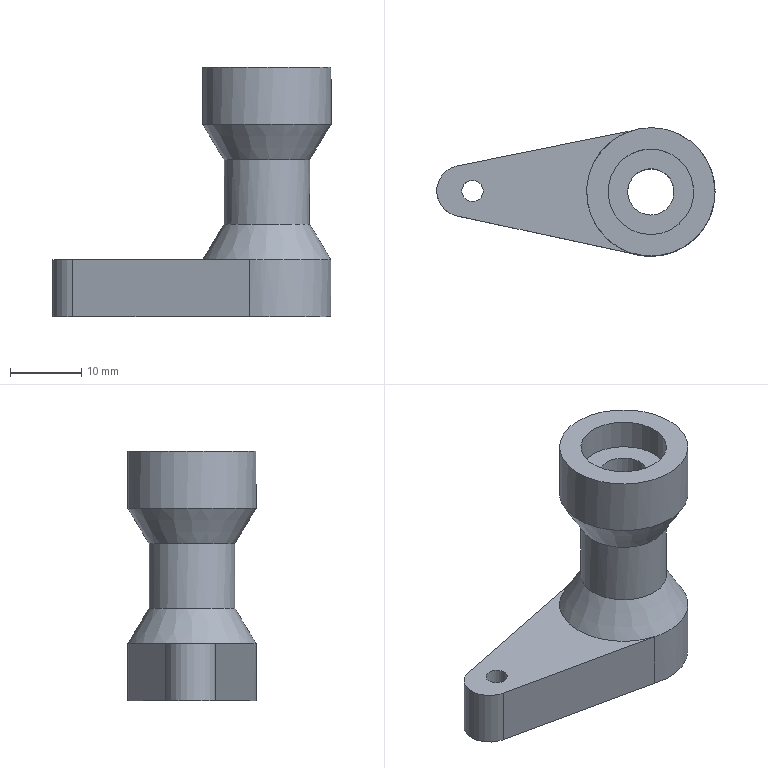Part | STEP file | Dodanie-wyci_gni_cie1_2 | 1 solid | 18 faces | box 38.999 x 17.999 x 35 mm | volume 6844 mm3 | cylinder 9 | plane 7 | cone 2 | commonest cylinder face diameters 11.999 x3 17.999 x3 3 x1 6.499 x1 7.151 x1
STEP:
#1=CARTESIAN_POINT('',(0.,0.,0.));
#2=DIRECTION('',(0.,0.,1.));
#3=DIRECTION('',(1.,0.,0.));
#4=AXIS2_PLACEMENT_3D('',#1,#2,#3);
#5=CARTESIAN_POINT('',(-38.722,78.388,-127.298));
#6=VERTEX_POINT('',#5);
#7=CARTESIAN_POINT('',(-38.744,75.138,-127.298));
#8=DIRECTION('',(0.,0.,1.));
#9=DIRECTION('',(0.006749,1.,0.));
#10=AXIS2_PLACEMENT_3D('',#7,#8,#9);
#11=CIRCLE('',#10,3.25);
#12=CARTESIAN_POINT('',(-38.744,75.138,-127.298));
#13=DIRECTION('',(0.,0.,1.));
#14=DIRECTION('',(0.006749,1.,0.));
#15=AXIS2_PLACEMENT_3D('',#12,#13,#14);
#16=CYLINDRICAL_SURFACE('',#15,3.25);
#17=CARTESIAN_POINT('',(0.,0.));
#18=DIRECTION('',(1.,0.));
#19=VECTOR('',#18,1.);
#20=LINE('',#17,#19);
#21=(GEOMETRIC_REPRESENTATION_CONTEXT(2)PARAMETRIC_REPRESENTATION_CONTEXT()REPRESENTATION_CONTEXT('',''));
#22=DEFINITIONAL_REPRESENTATION('',(#20),#21);
#23=PCURVE('',#16,#22);
#24=CARTESIAN_POINT('',(-38.744,75.138,-127.298));
#25=DIRECTION('',(0.,0.,-1.));
#26=DIRECTION('',(-0.006749,-1.,0.));
#27=AXIS2_PLACEMENT_3D('',#24,#25,#26);
#28=PLANE('',#27);
#29=CARTESIAN_POINT('',(-3.25,0.));
#30=CARTESIAN_POINT('',(-3.25,5.629));
#31=CARTESIAN_POINT('',(1.625,2.814));
#32=CARTESIAN_POINT('',(6.499,0.));
#33=CARTESIAN_POINT('',(1.625,-2.814));
#34=CARTESIAN_POINT('',(-3.25,-5.629));
#35=CARTESIAN_POINT('',(-3.25,0.));
#36=(BOUNDED_CURVE()B_SPLINE_CURVE(2,(#29,#30,#31,#32,#33,#34,#35),.UNSPECIFIED.,.T.,.F.)B_SPLINE_CURVE_WITH_KNOTS((1,2,2,2,2,1),(-2.094,0.,2.094,4.189,6.283,8.378),.UNSPECIFIED.)CURVE()GEOMETRIC_REPRESENTATION_ITEM()RATIONAL_B_SPLINE_CURVE((1.,0.5,1.,0.5,1.,0.5,1.))REPRESENTATION_ITEM(''));
#37=(GEOMETRIC_REPRESENTATION_CONTEXT(2)PARAMETRIC_REPRESENTATION_CONTEXT()REPRESENTATION_CONTEXT('',''));
#38=DEFINITIONAL_REPRESENTATION('',(#36),#37);
#39=PCURVE('',#28,#38);
#40=SURFACE_CURVE('',#11,(#23,#39),.PCURVE_S1.);
#41=EDGE_CURVE('',#6,#6,#40,.T.);
#42=ORIENTED_EDGE('',*,*,#41,.T.);
#43=CARTESIAN_POINT('',(-38.722,78.388,-100.698));
#44=VERTEX_POINT('',#43);
#45=CARTESIAN_POINT('',(-38.722,78.388,-100.698));
#46=DIRECTION('',(0.,0.,-1.));
#47=VECTOR('',#46,1.);
#48=LINE('',#45,#47);
#49=CARTESIAN_POINT('',(6.283,26.6));
#50=DIRECTION('',(0.,-1.));
#51=VECTOR('',#50,1.);
#52=LINE('',#49,#51);
#53=(GEOMETRIC_REPRESENTATION_CONTEXT(2)PARAMETRIC_REPRESENTATION_CONTEXT()REPRESENTATION_CONTEXT('',''));
#54=DEFINITIONAL_REPRESENTATION('',(#52),#53);
#55=PCURVE('',#16,#54);
#56=CARTESIAN_POINT('',(0.,26.6));
#57=DIRECTION('',(0.,-1.));
#58=VECTOR('',#57,1.);
#59=LINE('',#56,#58);
#60=(GEOMETRIC_REPRESENTATION_CONTEXT(2)PARAMETRIC_REPRESENTATION_CONTEXT()REPRESENTATION_CONTEXT('',''));
#61=DEFINITIONAL_REPRESENTATION('',(#59),#60);
#62=PCURVE('',#16,#61);
#63=SEAM_CURVE('',#48,(#55,#62),.PCURVE_S1.);
#64=EDGE_CURVE('',#44,#6,#63,.T.);
#65=ORIENTED_EDGE('',*,*,#64,.F.);
#66=CARTESIAN_POINT('',(-38.744,75.138,-100.698));
#67=DIRECTION('',(0.,0.,-1.));
#68=DIRECTION('',(0.006749,1.,0.));
#69=AXIS2_PLACEMENT_3D('',#66,#67,#68);
#70=CIRCLE('',#69,3.25);
#71=CARTESIAN_POINT('',(6.283,26.6));
#72=DIRECTION('',(-1.,0.));
#73=VECTOR('',#72,1.);
#74=LINE('',#71,#73);
#75=(GEOMETRIC_REPRESENTATION_CONTEXT(2)PARAMETRIC_REPRESENTATION_CONTEXT()REPRESENTATION_CONTEXT('',''));
#76=DEFINITIONAL_REPRESENTATION('',(#74),#75);
#77=PCURVE('',#16,#76);
#78=CARTESIAN_POINT('',(-38.744,75.138,-100.698));
#79=DIRECTION('',(0.,0.,-1.));
#80=DIRECTION('',(-0.006749,-1.,0.));
#81=AXIS2_PLACEMENT_3D('',#78,#79,#80);
#82=PLANE('',#81);
#83=CARTESIAN_POINT('',(0.,0.));
#84=DIRECTION('',(-1.,0.));
#85=AXIS2_PLACEMENT_2D('',#83,#84);
#86=CIRCLE('',#85,3.25);
#87=(GEOMETRIC_REPRESENTATION_CONTEXT(2)PARAMETRIC_REPRESENTATION_CONTEXT()REPRESENTATION_CONTEXT('',''));
#88=DEFINITIONAL_REPRESENTATION('',(#86),#87);
#89=PCURVE('',#82,#88);
#90=SURFACE_CURVE('',#70,(#77,#89),.PCURVE_S1.);
#91=EDGE_CURVE('',#44,#44,#90,.T.);
#92=ORIENTED_EDGE('',*,*,#91,.T.);
#93=ORIENTED_EDGE('',*,*,#64,.T.);
#94=EDGE_LOOP('',(#42,#65,#92,#93));
#95=FACE_BOUND('',#94,.F.);
#96=ADVANCED_FACE('',(#95),#16,.F.);
#97=CARTESIAN_POINT('',(-38.704,81.138,-131.498));
#98=VERTEX_POINT('',#97);
#99=CARTESIAN_POINT('',(-38.744,75.138,-131.498));
#100=DIRECTION('',(0.,0.,1.));
#101=DIRECTION('',(0.006749,1.,0.));
#102=AXIS2_PLACEMENT_3D('',#99,#100,#101);
#103=CIRCLE('',#102,6.);
#104=CARTESIAN_POINT('',(-38.744,75.138,-131.498));
#105=DIRECTION('',(0.,0.,1.));
#106=DIRECTION('',(0.006749,1.,0.));
#107=AXIS2_PLACEMENT_3D('',#104,#105,#106);
#108=CYLINDRICAL_SURFACE('',#107,6.);
#109=CARTESIAN_POINT('',(0.,0.));
#110=DIRECTION('',(1.,0.));
#111=VECTOR('',#110,1.);
#112=LINE('',#109,#111);
#113=(GEOMETRIC_REPRESENTATION_CONTEXT(2)PARAMETRIC_REPRESENTATION_CONTEXT()REPRESENTATION_CONTEXT('',''));
#114=DEFINITIONAL_REPRESENTATION('',(#112),#113);
#115=PCURVE('',#108,#114);
#116=CARTESIAN_POINT('',(-49.244,75.209,-131.498));
#117=DIRECTION('',(0.,0.,-1.));
#118=DIRECTION('',(-0.006749,-1.,0.));
#119=AXIS2_PLACEMENT_3D('',#116,#117,#118);
#120=PLANE('',#119);
#121=CARTESIAN_POINT('',(-6.,-10.5));
#122=CARTESIAN_POINT('',(-6.,-0.1086));
#123=CARTESIAN_POINT('',(3.,-5.304));
#124=CARTESIAN_POINT('',(11.999,-10.5));
#125=CARTESIAN_POINT('',(3.,-15.696));
#126=CARTESIAN_POINT('',(-6.,-20.892));
#127=CARTESIAN_POINT('',(-6.,-10.5));
#128=(BOUNDED_CURVE()B_SPLINE_CURVE(2,(#121,#122,#123,#124,#125,#126,#127),.UNSPECIFIED.,.T.,.F.)B_SPLINE_CURVE_WITH_KNOTS((1,2,2,2,2,1),(-2.094,0.,2.094,4.189,6.283,8.378),.UNSPECIFIED.)CURVE()GEOMETRIC_REPRESENTATION_ITEM()RATIONAL_B_SPLINE_CURVE((1.,0.5,1.,0.5,1.,0.5,1.))REPRESENTATION_ITEM(''));
#129=(GEOMETRIC_REPRESENTATION_CONTEXT(2)PARAMETRIC_REPRESENTATION_CONTEXT()REPRESENTATION_CONTEXT('',''));
#130=DEFINITIONAL_REPRESENTATION('',(#128),#129);
#131=PCURVE('',#120,#130);
#132=SURFACE_CURVE('',#103,(#115,#131),.PCURVE_S1.);
#133=EDGE_CURVE('',#98,#98,#132,.T.);
#134=ORIENTED_EDGE('',*,*,#133,.T.);
#135=CARTESIAN_POINT('',(-38.704,81.138,-127.298));
#136=VERTEX_POINT('',#135);
#137=CARTESIAN_POINT('',(-38.704,81.138,-127.298));
#138=DIRECTION('',(0.,0.,-1.));
#139=VECTOR('',#138,1.);
#140=LINE('',#137,#139);
#141=CARTESIAN_POINT('',(6.283,4.2));
#142=DIRECTION('',(0.,-1.));
#143=VECTOR('',#142,1.);
#144=LINE('',#141,#143);
#145=(GEOMETRIC_REPRESENTATION_CONTEXT(2)PARAMETRIC_REPRESENTATION_CONTEXT()REPRESENTATION_CONTEXT('',''));
#146=DEFINITIONAL_REPRESENTATION('',(#144),#145);
#147=PCURVE('',#108,#146);
#148=CARTESIAN_POINT('',(0.,4.2));
#149=DIRECTION('',(0.,-1.));
#150=VECTOR('',#149,1.);
#151=LINE('',#148,#150);
#152=(GEOMETRIC_REPRESENTATION_CONTEXT(2)PARAMETRIC_REPRESENTATION_CONTEXT()REPRESENTATION_CONTEXT('',''));
#153=DEFINITIONAL_REPRESENTATION('',(#151),#152);
#154=PCURVE('',#108,#153);
#155=SEAM_CURVE('',#140,(#147,#154),.PCURVE_S1.);
#156=EDGE_CURVE('',#136,#98,#155,.T.);
#157=ORIENTED_EDGE('',*,*,#156,.F.);
#158=CARTESIAN_POINT('',(-38.744,75.138,-127.298));
#159=DIRECTION('',(0.,0.,-1.));
#160=DIRECTION('',(0.006749,1.,0.));
#161=AXIS2_PLACEMENT_3D('',#158,#159,#160);
#162=CIRCLE('',#161,6.);
#163=CARTESIAN_POINT('',(6.283,4.2));
#164=DIRECTION('',(-1.,0.));
#165=VECTOR('',#164,1.);
#166=LINE('',#163,#165);
#167=(GEOMETRIC_REPRESENTATION_CONTEXT(2)PARAMETRIC_REPRESENTATION_CONTEXT()REPRESENTATION_CONTEXT('',''));
#168=DEFINITIONAL_REPRESENTATION('',(#166),#167);
#169=PCURVE('',#108,#168);
#170=CARTESIAN_POINT('',(0.,0.));
#171=DIRECTION('',(-1.,0.));
#172=AXIS2_PLACEMENT_2D('',#170,#171);
#173=CIRCLE('',#172,6.);
#174=(GEOMETRIC_REPRESENTATION_CONTEXT(2)PARAMETRIC_REPRESENTATION_CONTEXT()REPRESENTATION_CONTEXT('',''));
#175=DEFINITIONAL_REPRESENTATION('',(#173),#174);
#176=PCURVE('',#28,#175);
#177=SURFACE_CURVE('',#162,(#169,#176),.PCURVE_S1.);
#178=EDGE_CURVE('',#136,#136,#177,.T.);
#179=ORIENTED_EDGE('',*,*,#178,.T.);
#180=ORIENTED_EDGE('',*,*,#156,.T.);
#181=EDGE_LOOP('',(#134,#157,#179,#180));
#182=FACE_BOUND('',#181,.F.);
#183=ADVANCED_FACE('',(#182),#108,.F.);
#184=CARTESIAN_POINT('',(-38.704,81.138,-100.698));
#185=VERTEX_POINT('',#184);
#186=CARTESIAN_POINT('',(-38.744,75.138,-100.698));
#187=DIRECTION('',(0.,0.,-1.));
#188=DIRECTION('',(0.006749,1.,0.));
#189=AXIS2_PLACEMENT_3D('',#186,#187,#188);
#190=CIRCLE('',#189,6.);
#191=CARTESIAN_POINT('',(-38.744,75.138,-100.698));
#192=DIRECTION('',(0.,0.,1.));
#193=DIRECTION('',(0.006749,1.,0.));
#194=AXIS2_PLACEMENT_3D('',#191,#192,#193);
#195=CYLINDRICAL_SURFACE('',#194,6.);
#196=CARTESIAN_POINT('',(6.283,0.));
#197=DIRECTION('',(-1.,0.));
#198=VECTOR('',#197,1.);
#199=LINE('',#196,#198);
#200=(GEOMETRIC_REPRESENTATION_CONTEXT(2)PARAMETRIC_REPRESENTATION_CONTEXT()REPRESENTATION_CONTEXT('',''));
#201=DEFINITIONAL_REPRESENTATION('',(#199),#200);
#202=PCURVE('',#195,#201);
#203=CARTESIAN_POINT('',(0.,0.));
#204=DIRECTION('',(-1.,0.));
#205=AXIS2_PLACEMENT_2D('',#203,#204);
#206=CIRCLE('',#205,6.);
#207=(GEOMETRIC_REPRESENTATION_CONTEXT(2)PARAMETRIC_REPRESENTATION_CONTEXT()REPRESENTATION_CONTEXT('',''));
#208=DEFINITIONAL_REPRESENTATION('',(#206),#207);
#209=PCURVE('',#82,#208);
#210=SURFACE_CURVE('',#190,(#202,#209),.PCURVE_S1.);
#211=EDGE_CURVE('',#185,#185,#210,.T.);
#212=ORIENTED_EDGE('',*,*,#211,.F.);
#213=CARTESIAN_POINT('',(-38.704,81.138,-96.498));
#214=VERTEX_POINT('',#213);
#215=CARTESIAN_POINT('',(-38.704,81.138,-96.498));
#216=DIRECTION('',(0.,0.,-1.));
#217=VECTOR('',#216,1.);
#218=LINE('',#215,#217);
#219=CARTESIAN_POINT('',(6.283,4.2));
#220=DIRECTION('',(0.,-1.));
#221=VECTOR('',#220,1.);
#222=LINE('',#219,#221);
#223=(GEOMETRIC_REPRESENTATION_CONTEXT(2)PARAMETRIC_REPRESENTATION_CONTEXT()REPRESENTATION_CONTEXT('',''));
#224=DEFINITIONAL_REPRESENTATION('',(#222),#223);
#225=PCURVE('',#195,#224);
#226=CARTESIAN_POINT('',(0.,4.2));
#227=DIRECTION('',(0.,-1.));
#228=VECTOR('',#227,1.);
#229=LINE('',#226,#228);
#230=(GEOMETRIC_REPRESENTATION_CONTEXT(2)PARAMETRIC_REPRESENTATION_CONTEXT()REPRESENTATION_CONTEXT('',''));
#231=DEFINITIONAL_REPRESENTATION('',(#229),#230);
#232=PCURVE('',#195,#231);
#233=SEAM_CURVE('',#218,(#225,#232),.PCURVE_S1.);
#234=EDGE_CURVE('',#214,#185,#233,.T.);
#235=ORIENTED_EDGE('',*,*,#234,.F.);
#236=CARTESIAN_POINT('',(-38.744,75.138,-96.498));
#237=DIRECTION('',(0.,0.,-1.));
#238=DIRECTION('',(0.006749,1.,0.));
#239=AXIS2_PLACEMENT_3D('',#236,#237,#238);
#240=CIRCLE('',#239,6.);
#241=CARTESIAN_POINT('',(6.283,4.2));
#242=DIRECTION('',(-1.,0.));
#243=VECTOR('',#242,1.);
#244=LINE('',#241,#243);
#245=(GEOMETRIC_REPRESENTATION_CONTEXT(2)PARAMETRIC_REPRESENTATION_CONTEXT()REPRESENTATION_CONTEXT('',''));
#246=DEFINITIONAL_REPRESENTATION('',(#244),#245);
#247=PCURVE('',#195,#246);
#248=CARTESIAN_POINT('',(-38.744,75.138,-96.498));
#249=DIRECTION('',(0.,0.,1.));
#250=DIRECTION('',(0.006749,1.,0.));
#251=AXIS2_PLACEMENT_3D('',#248,#249,#250);
#252=PLANE('',#251);
#253=CARTESIAN_POINT('',(6.,0.));
#254=CARTESIAN_POINT('',(6.,-10.392));
#255=CARTESIAN_POINT('',(-3.,-5.196));
#256=CARTESIAN_POINT('',(-11.999,0.));
#257=CARTESIAN_POINT('',(-3.,5.196));
#258=CARTESIAN_POINT('',(6.,10.392));
#259=CARTESIAN_POINT('',(6.,0.));
#260=(BOUNDED_CURVE()B_SPLINE_CURVE(2,(#253,#254,#255,#256,#257,#258,#259),.UNSPECIFIED.,.T.,.F.)B_SPLINE_CURVE_WITH_KNOTS((1,2,2,2,2,1),(-2.094,0.,2.094,4.189,6.283,8.378),.UNSPECIFIED.)CURVE()GEOMETRIC_REPRESENTATION_ITEM()RATIONAL_B_SPLINE_CURVE((1.,0.5,1.,0.5,1.,0.5,1.))REPRESENTATION_ITEM(''));
#261=(GEOMETRIC_REPRESENTATION_CONTEXT(2)PARAMETRIC_REPRESENTATION_CONTEXT()REPRESENTATION_CONTEXT('',''));
#262=DEFINITIONAL_REPRESENTATION('',(#260),#261);
#263=PCURVE('',#252,#262);
#264=SURFACE_CURVE('',#240,(#247,#263),.PCURVE_S1.);
#265=EDGE_CURVE('',#214,#214,#264,.T.);
#266=ORIENTED_EDGE('',*,*,#265,.T.);
#267=ORIENTED_EDGE('',*,*,#234,.T.);
#268=EDGE_LOOP('',(#212,#235,#266,#267));
#269=FACE_BOUND('',#268,.F.);
#270=ADVANCED_FACE('',(#269),#195,.F.);
#271=CARTESIAN_POINT('',(-63.754,73.807,-123.498));
#272=VERTEX_POINT('',#271);
#273=CARTESIAN_POINT('',(-63.744,75.307,-123.498));
#274=DIRECTION('',(0.,0.,-1.));
#275=DIRECTION('',(-0.006749,-1.,0.));
#276=AXIS2_PLACEMENT_3D('',#273,#274,#275);
#277=CIRCLE('',#276,1.5);
#278=CARTESIAN_POINT('',(-63.744,75.307,-123.498));
#279=DIRECTION('',(0.,0.,-1.));
#280=DIRECTION('',(-0.006749,-1.,0.));
#281=AXIS2_PLACEMENT_3D('',#278,#279,#280);
#282=CYLINDRICAL_SURFACE('',#281,1.5);
#283=CARTESIAN_POINT('',(0.,0.));
#284=DIRECTION('',(1.,0.));
#285=VECTOR('',#284,1.);
#286=LINE('',#283,#285);
#287=(GEOMETRIC_REPRESENTATION_CONTEXT(2)PARAMETRIC_REPRESENTATION_CONTEXT()REPRESENTATION_CONTEXT('',''));
#288=DEFINITIONAL_REPRESENTATION('',(#286),#287);
#289=PCURVE('',#282,#288);
#290=CARTESIAN_POINT('',(-54.951,75.248,-123.498));
#291=DIRECTION('',(0.,0.,1.));
#292=DIRECTION('',(0.006749,1.,0.));
#293=AXIS2_PLACEMENT_3D('',#290,#291,#292);
#294=PLANE('',#293);
#295=CARTESIAN_POINT('',(-1.5,8.793));
#296=CARTESIAN_POINT('',(-1.5,11.391));
#297=CARTESIAN_POINT('',(0.75,10.092));
#298=CARTESIAN_POINT('',(3.,8.793));
#299=CARTESIAN_POINT('',(0.75,7.494));
#300=CARTESIAN_POINT('',(-1.5,6.195));
#301=CARTESIAN_POINT('',(-1.5,8.793));
#302=(BOUNDED_CURVE()B_SPLINE_CURVE(2,(#295,#296,#297,#298,#299,#300,#301),.UNSPECIFIED.,.T.,.F.)B_SPLINE_CURVE_WITH_KNOTS((1,2,2,2,2,1),(-2.094,0.,2.094,4.189,6.283,8.378),.UNSPECIFIED.)CURVE()GEOMETRIC_REPRESENTATION_ITEM()RATIONAL_B_SPLINE_CURVE((1.,0.5,1.,0.5,1.,0.5,1.))REPRESENTATION_ITEM(''));
#303=(GEOMETRIC_REPRESENTATION_CONTEXT(2)PARAMETRIC_REPRESENTATION_CONTEXT()REPRESENTATION_CONTEXT('',''));
#304=DEFINITIONAL_REPRESENTATION('',(#302),#303);
#305=PCURVE('',#294,#304);
#306=SURFACE_CURVE('',#277,(#289,#305),.PCURVE_S1.);
#307=EDGE_CURVE('',#272,#272,#306,.T.);
#308=ORIENTED_EDGE('',*,*,#307,.T.);
#309=CARTESIAN_POINT('',(-63.754,73.807,-131.498));
#310=VERTEX_POINT('',#309);
#311=CARTESIAN_POINT('',(-63.754,73.807,-131.498));
#312=DIRECTION('',(0.,0.,1.));
#313=VECTOR('',#312,1.);
#314=LINE('',#311,#313);
#315=CARTESIAN_POINT('',(6.283,8.));
#316=DIRECTION('',(0.,-1.));
#317=VECTOR('',#316,1.);
#318=LINE('',#315,#317);
#319=(GEOMETRIC_REPRESENTATION_CONTEXT(2)PARAMETRIC_REPRESENTATION_CONTEXT()REPRESENTATION_CONTEXT('',''));
#320=DEFINITIONAL_REPRESENTATION('',(#318),#319);
#321=PCURVE('',#282,#320);
#322=CARTESIAN_POINT('',(0.,8.));
#323=DIRECTION('',(0.,-1.));
#324=VECTOR('',#323,1.);
#325=LINE('',#322,#324);
#326=(GEOMETRIC_REPRESENTATION_CONTEXT(2)PARAMETRIC_REPRESENTATION_CONTEXT()REPRESENTATION_CONTEXT('',''));
#327=DEFINITIONAL_REPRESENTATION('',(#325),#326);
#328=PCURVE('',#282,#327);
#329=SEAM_CURVE('',#314,(#321,#328),.PCURVE_S1.);
#330=EDGE_CURVE('',#310,#272,#329,.T.);
#331=ORIENTED_EDGE('',*,*,#330,.F.);
#332=CARTESIAN_POINT('',(-63.744,75.307,-131.498));
#333=DIRECTION('',(0.,0.,1.));
#334=DIRECTION('',(-0.006749,-1.,0.));
#335=AXIS2_PLACEMENT_3D('',#332,#333,#334);
#336=CIRCLE('',#335,1.5);
#337=CARTESIAN_POINT('',(6.283,8.));
#338=DIRECTION('',(-1.,0.));
#339=VECTOR('',#338,1.);
#340=LINE('',#337,#339);
#341=(GEOMETRIC_REPRESENTATION_CONTEXT(2)PARAMETRIC_REPRESENTATION_CONTEXT()REPRESENTATION_CONTEXT('',''));
#342=DEFINITIONAL_REPRESENTATION('',(#340),#341);
#343=PCURVE('',#282,#342);
#344=CARTESIAN_POINT('',(1.5,14.5));
#345=CARTESIAN_POINT('',(1.5,11.902));
#346=CARTESIAN_POINT('',(-0.75,13.201));
#347=CARTESIAN_POINT('',(-3.,14.5));
#348=CARTESIAN_POINT('',(-0.75,15.799));
#349=CARTESIAN_POINT('',(1.5,17.098));
#350=CARTESIAN_POINT('',(1.5,14.5));
#351=(BOUNDED_CURVE()B_SPLINE_CURVE(2,(#344,#345,#346,#347,#348,#349,#350),.UNSPECIFIED.,.T.,.F.)B_SPLINE_CURVE_WITH_KNOTS((1,2,2,2,2,1),(-2.094,0.,2.094,4.189,6.283,8.378),.UNSPECIFIED.)CURVE()GEOMETRIC_REPRESENTATION_ITEM()RATIONAL_B_SPLINE_CURVE((1.,0.5,1.,0.5,1.,0.5,1.))REPRESENTATION_ITEM(''));
#352=(GEOMETRIC_REPRESENTATION_CONTEXT(2)PARAMETRIC_REPRESENTATION_CONTEXT()REPRESENTATION_CONTEXT('',''));
#353=DEFINITIONAL_REPRESENTATION('',(#351),#352);
#354=PCURVE('',#120,#353);
#355=SURFACE_CURVE('',#336,(#343,#354),.PCURVE_S1.);
#356=EDGE_CURVE('',#310,#310,#355,.T.);
#357=ORIENTED_EDGE('',*,*,#356,.T.);
#358=ORIENTED_EDGE('',*,*,#330,.T.);
#359=EDGE_LOOP('',(#308,#331,#357,#358));
#360=FACE_BOUND('',#359,.F.);
#361=ADVANCED_FACE('',(#360),#282,.F.);
#362=CARTESIAN_POINT('',(-38.684,84.138,-123.498));
#363=VERTEX_POINT('',#362);
#364=CARTESIAN_POINT('',(-38.684,84.138,-131.498));
#365=VERTEX_POINT('',#364);
#366=CARTESIAN_POINT('',(-38.684,84.138,-123.498));
#367=DIRECTION('',(0.,0.,-1.));
#368=VECTOR('',#367,1.);
#369=LINE('',#366,#368);
#370=CARTESIAN_POINT('',(-38.744,75.138,-131.498));
#371=DIRECTION('',(0.,0.,1.));
#372=DIRECTION('',(0.006749,1.,0.));
#373=AXIS2_PLACEMENT_3D('',#370,#371,#372);
#374=CYLINDRICAL_SURFACE('',#373,9.);
#375=CARTESIAN_POINT('',(0.,8.));
#376=DIRECTION('',(0.,-1.));
#377=VECTOR('',#376,1.);
#378=LINE('',#375,#377);
#379=(GEOMETRIC_REPRESENTATION_CONTEXT(2)PARAMETRIC_REPRESENTATION_CONTEXT()REPRESENTATION_CONTEXT('',''));
#380=DEFINITIONAL_REPRESENTATION('',(#378),#379);
#381=PCURVE('',#374,#380);
#382=CARTESIAN_POINT('',(-38.744,75.138,-131.498));
#383=DIRECTION('',(0.,0.,1.));
#384=DIRECTION('',(0.006749,1.,0.));
#385=AXIS2_PLACEMENT_3D('',#382,#383,#384);
#386=CYLINDRICAL_SURFACE('',#385,9.);
#387=CARTESIAN_POINT('',(6.283,8.));
#388=DIRECTION('',(0.,-1.));
#389=VECTOR('',#388,1.);
#390=LINE('',#387,#389);
#391=(GEOMETRIC_REPRESENTATION_CONTEXT(2)PARAMETRIC_REPRESENTATION_CONTEXT()REPRESENTATION_CONTEXT('',''));
#392=DEFINITIONAL_REPRESENTATION('',(#390),#391);
#393=PCURVE('',#386,#392);
#394=SURFACE_CURVE('',#369,(#381,#393),.PCURVE_S1.);
#395=EDGE_CURVE('',#363,#365,#394,.T.);
#396=ORIENTED_EDGE('',*,*,#395,.T.);
#397=CARTESIAN_POINT('',(-41.1,83.824,-131.498));
#398=VERTEX_POINT('',#397);
#399=CARTESIAN_POINT('',(-38.744,75.138,-131.498));
#400=DIRECTION('',(0.,0.,-1.));
#401=DIRECTION('',(0.006749,1.,0.));
#402=AXIS2_PLACEMENT_3D('',#399,#400,#401);
#403=CIRCLE('',#402,9.);
#404=CARTESIAN_POINT('',(6.283,0.));
#405=DIRECTION('',(-1.,0.));
#406=VECTOR('',#405,1.);
#407=LINE('',#404,#406);
#408=(GEOMETRIC_REPRESENTATION_CONTEXT(2)PARAMETRIC_REPRESENTATION_CONTEXT()REPRESENTATION_CONTEXT('',''));
#409=DEFINITIONAL_REPRESENTATION('',(#407),#408);
#410=PCURVE('',#374,#409);
#411=CARTESIAN_POINT('',(-0.000000004,-10.5));
#412=DIRECTION('',(-1.,0.));
#413=AXIS2_PLACEMENT_2D('',#411,#412);
#414=CIRCLE('',#413,9.);
#415=(GEOMETRIC_REPRESENTATION_CONTEXT(2)PARAMETRIC_REPRESENTATION_CONTEXT()REPRESENTATION_CONTEXT('',''));
#416=DEFINITIONAL_REPRESENTATION('',(#414),#415);
#417=PCURVE('',#120,#416);
#418=SURFACE_CURVE('',#403,(#410,#417),.PCURVE_S1.);
#419=EDGE_CURVE('',#398,#365,#418,.T.);
#420=ORIENTED_EDGE('',*,*,#419,.F.);
#421=CARTESIAN_POINT('',(-41.1,83.824,-123.498));
#422=VERTEX_POINT('',#421);
#423=CARTESIAN_POINT('',(-41.1,83.824,-123.498));
#424=DIRECTION('',(0.,0.,-1.));
#425=VECTOR('',#424,1.);
#426=LINE('',#423,#425);
#427=CARTESIAN_POINT('',(0.2716,8.));
#428=DIRECTION('',(0.,-1.));
#429=VECTOR('',#428,1.);
#430=LINE('',#427,#429);
#431=(GEOMETRIC_REPRESENTATION_CONTEXT(2)PARAMETRIC_REPRESENTATION_CONTEXT()REPRESENTATION_CONTEXT('',''));
#432=DEFINITIONAL_REPRESENTATION('',(#430),#431);
#433=PCURVE('',#374,#432);
#434=CARTESIAN_POINT('',(-53.488,81.323,-127.498));
#435=DIRECTION('',(-0.1979,0.9802,0.));
#436=DIRECTION('',(0.9802,0.1979,0.));
#437=AXIS2_PLACEMENT_3D('',#434,#435,#436);
#438=PLANE('',#437);
#439=CARTESIAN_POINT('',(12.638,-4.));
#440=DIRECTION('',(0.,1.));
#441=VECTOR('',#440,1.);
#442=LINE('',#439,#441);
#443=(GEOMETRIC_REPRESENTATION_CONTEXT(2)PARAMETRIC_REPRESENTATION_CONTEXT()REPRESENTATION_CONTEXT('',''));
#444=DEFINITIONAL_REPRESENTATION('',(#442),#443);
#445=PCURVE('',#438,#444);
#446=SURFACE_CURVE('',#426,(#433,#445),.PCURVE_S1.);
#447=EDGE_CURVE('',#422,#398,#446,.T.);
#448=ORIENTED_EDGE('',*,*,#447,.F.);
#449=CARTESIAN_POINT('',(-38.744,75.138,-123.498));
#450=DIRECTION('',(0.,0.,-1.));
#451=DIRECTION('',(0.006749,1.,0.));
#452=AXIS2_PLACEMENT_3D('',#449,#450,#451);
#453=CIRCLE('',#452,9.);
#454=CARTESIAN_POINT('',(6.283,8.));
#455=DIRECTION('',(-1.,0.));
#456=VECTOR('',#455,1.);
#457=LINE('',#454,#456);
#458=(GEOMETRIC_REPRESENTATION_CONTEXT(2)PARAMETRIC_REPRESENTATION_CONTEXT()REPRESENTATION_CONTEXT('',''));
#459=DEFINITIONAL_REPRESENTATION('',(#457),#458);
#460=PCURVE('',#374,#459);
#461=CARTESIAN_POINT('',(-38.744,75.138,-123.498));
#462=DIRECTION('',(0.,0.,-1.));
#463=DIRECTION('',(-0.006749,-1.,0.));
#464=AXIS2_PLACEMENT_3D('',#461,#462,#463);
#465=CONICAL_SURFACE('',#464,9.,0.5404);
#466=CARTESIAN_POINT('',(-3.142,0.));
#467=DIRECTION('',(1.,0.));
#468=VECTOR('',#467,1.);
#469=LINE('',#466,#468);
#470=(GEOMETRIC_REPRESENTATION_CONTEXT(2)PARAMETRIC_REPRESENTATION_CONTEXT()REPRESENTATION_CONTEXT('',''));
#471=DEFINITIONAL_REPRESENTATION('',(#469),#470);
#472=PCURVE('',#465,#471);
#473=SURFACE_CURVE('',#453,(#460,#472),.PCURVE_S1.);
#474=EDGE_CURVE('',#422,#363,#473,.T.);
#475=ORIENTED_EDGE('',*,*,#474,.T.);
#476=EDGE_LOOP('',(#396,#420,#448,#475));
#477=FACE_BOUND('',#476,.T.);
#478=ADVANCED_FACE('',(#477),#374,.T.);
#479=CARTESIAN_POINT('',(-38.684,84.138,-96.498));
#480=VERTEX_POINT('',#479);
#481=CARTESIAN_POINT('',(-38.684,84.138,-104.498));
#482=VERTEX_POINT('',#481);
#483=CARTESIAN_POINT('',(-38.684,84.138,-96.498));
#484=DIRECTION('',(0.,0.,-1.));
#485=VECTOR('',#484,1.);
#486=LINE('',#483,#485);
#487=CARTESIAN_POINT('',(-38.744,75.138,-104.498));
#488=DIRECTION('',(0.,0.,1.));
#489=DIRECTION('',(0.006749,1.,0.));
#490=AXIS2_PLACEMENT_3D('',#487,#488,#489);
#491=CYLINDRICAL_SURFACE('',#490,9.);
#492=CARTESIAN_POINT('',(0.,8.));
#493=DIRECTION('',(0.,-1.));
#494=VECTOR('',#493,1.);
#495=LINE('',#492,#494);
#496=(GEOMETRIC_REPRESENTATION_CONTEXT(2)PARAMETRIC_REPRESENTATION_CONTEXT()REPRESENTATION_CONTEXT('',''));
#497=DEFINITIONAL_REPRESENTATION('',(#495),#496);
#498=PCURVE('',#491,#497);
#499=CARTESIAN_POINT('',(6.283,8.));
#500=DIRECTION('',(0.,-1.));
#501=VECTOR('',#500,1.);
#502=LINE('',#499,#501);
#503=(GEOMETRIC_REPRESENTATION_CONTEXT(2)PARAMETRIC_REPRESENTATION_CONTEXT()REPRESENTATION_CONTEXT('',''));
#504=DEFINITIONAL_REPRESENTATION('',(#502),#503);
#505=PCURVE('',#491,#504);
#506=SEAM_CURVE('',#486,(#498,#505),.PCURVE_S1.);
#507=EDGE_CURVE('',#480,#482,#506,.T.);
#508=ORIENTED_EDGE('',*,*,#507,.T.);
#509=CARTESIAN_POINT('',(-29.745,75.077,-104.498));
#510=VERTEX_POINT('',#509);
#511=CARTESIAN_POINT('',(-38.744,75.138,-104.498));
#512=DIRECTION('',(0.,0.,1.));
#513=DIRECTION('',(0.006749,1.,0.));
#514=AXIS2_PLACEMENT_3D('',#511,#512,#513);
#515=CIRCLE('',#514,9.);
#516=CARTESIAN_POINT('',(0.,0.));
#517=DIRECTION('',(1.,0.));
#518=VECTOR('',#517,1.);
#519=LINE('',#516,#518);
#520=(GEOMETRIC_REPRESENTATION_CONTEXT(2)PARAMETRIC_REPRESENTATION_CONTEXT()REPRESENTATION_CONTEXT('',''));
#521=DEFINITIONAL_REPRESENTATION('',(#519),#520);
#522=PCURVE('',#491,#521);
#523=CARTESIAN_POINT('',(-38.744,75.138,-104.498));
#524=DIRECTION('',(0.,0.,1.));
#525=DIRECTION('',(1.,-0.006749,0.));
#526=AXIS2_PLACEMENT_3D('',#523,#524,#525);
#527=CONICAL_SURFACE('',#526,9.,0.5404);
#528=CARTESIAN_POINT('',(1.571,0.));
#529=DIRECTION('',(1.,0.));
#530=VECTOR('',#529,1.);
#531=LINE('',#528,#530);
#532=(GEOMETRIC_REPRESENTATION_CONTEXT(2)PARAMETRIC_REPRESENTATION_CONTEXT()REPRESENTATION_CONTEXT('',''));
#533=DEFINITIONAL_REPRESENTATION('',(#531),#532);
#534=PCURVE('',#527,#533);
#535=SURFACE_CURVE('',#515,(#522,#534),.PCURVE_S1.);
#536=EDGE_CURVE('',#482,#510,#535,.T.);
#537=ORIENTED_EDGE('',*,*,#536,.T.);
#538=CARTESIAN_POINT('',(-38.744,75.138,-104.498));
#539=DIRECTION('',(0.,0.,1.));
#540=DIRECTION('',(0.006749,1.,0.));
#541=AXIS2_PLACEMENT_3D('',#538,#539,#540);
#542=CIRCLE('',#541,9.);
#543=CARTESIAN_POINT('',(0.,0.));
#544=DIRECTION('',(1.,0.));
#545=VECTOR('',#544,1.);
#546=LINE('',#543,#545);
#547=(GEOMETRIC_REPRESENTATION_CONTEXT(2)PARAMETRIC_REPRESENTATION_CONTEXT()REPRESENTATION_CONTEXT('',''));
#548=DEFINITIONAL_REPRESENTATION('',(#546),#547);
#549=PCURVE('',#491,#548);
#550=CARTESIAN_POINT('',(-4.712,0.));
#551=DIRECTION('',(1.,0.));
#552=VECTOR('',#551,1.);
#553=LINE('',#550,#552);
#554=(GEOMETRIC_REPRESENTATION_CONTEXT(2)PARAMETRIC_REPRESENTATION_CONTEXT()REPRESENTATION_CONTEXT('',''));
#555=DEFINITIONAL_REPRESENTATION('',(#553),#554);
#556=PCURVE('',#527,#555);
#557=SURFACE_CURVE('',#542,(#549,#556),.PCURVE_S1.);
#558=EDGE_CURVE('',#510,#482,#557,.T.);
#559=ORIENTED_EDGE('',*,*,#558,.T.);
#560=ORIENTED_EDGE('',*,*,#507,.F.);
#561=CARTESIAN_POINT('',(-38.744,75.138,-96.498));
#562=DIRECTION('',(0.,0.,1.));
#563=DIRECTION('',(0.006749,1.,0.));
#564=AXIS2_PLACEMENT_3D('',#561,#562,#563);
#565=CIRCLE('',#564,9.);
#566=CARTESIAN_POINT('',(0.,8.));
#567=DIRECTION('',(1.,0.));
#568=VECTOR('',#567,1.);
#569=LINE('',#566,#568);
#570=(GEOMETRIC_REPRESENTATION_CONTEXT(2)PARAMETRIC_REPRESENTATION_CONTEXT()REPRESENTATION_CONTEXT('',''));
#571=DEFINITIONAL_REPRESENTATION('',(#569),#570);
#572=PCURVE('',#491,#571);
#573=CARTESIAN_POINT('',(0.,0.));
#574=DIRECTION('',(1.,0.));
#575=AXIS2_PLACEMENT_2D('',#573,#574);
#576=CIRCLE('',#575,9.);
#577=(GEOMETRIC_REPRESENTATION_CONTEXT(2)PARAMETRIC_REPRESENTATION_CONTEXT()REPRESENTATION_CONTEXT('',''));
#578=DEFINITIONAL_REPRESENTATION('',(#576),#577);
#579=PCURVE('',#252,#578);
#580=SURFACE_CURVE('',#565,(#572,#579),.PCURVE_S1.);
#581=EDGE_CURVE('',#480,#480,#580,.T.);
#582=ORIENTED_EDGE('',*,*,#581,.F.);
#583=EDGE_LOOP('',(#508,#537,#559,#560,#582));
#584=FACE_BOUND('',#583,.T.);
#585=ADVANCED_FACE('',(#584),#491,.T.);
#586=CARTESIAN_POINT('',(-38.805,66.139,-123.498));
#587=VERTEX_POINT('',#586);
#588=CARTESIAN_POINT('',(-38.785,69.139,-118.498));
#589=VERTEX_POINT('',#588);
#590=CARTESIAN_POINT('',(-38.805,66.139,-123.498));
#591=DIRECTION('',(0.003472,0.5145,0.8575));
#592=VECTOR('',#591,1.);
#593=LINE('',#590,#592);
#594=CARTESIAN_POINT('',(0.,0.));
#595=DIRECTION('',(0.,-1.));
#596=VECTOR('',#595,1.);
#597=LINE('',#594,#596);
#598=(GEOMETRIC_REPRESENTATION_CONTEXT(2)PARAMETRIC_REPRESENTATION_CONTEXT()REPRESENTATION_CONTEXT('',''));
#599=DEFINITIONAL_REPRESENTATION('',(#597),#598);
#600=PCURVE('',#465,#599);
#601=CARTESIAN_POINT('',(6.283,0.));
#602=DIRECTION('',(0.,-1.));
#603=VECTOR('',#602,1.);
#604=LINE('',#601,#603);
#605=(GEOMETRIC_REPRESENTATION_CONTEXT(2)PARAMETRIC_REPRESENTATION_CONTEXT()REPRESENTATION_CONTEXT('',''));
#606=DEFINITIONAL_REPRESENTATION('',(#604),#605);
#607=PCURVE('',#465,#606);
#608=SEAM_CURVE('',#593,(#600,#607),.PCURVE_S1.);
#609=EDGE_CURVE('',#587,#589,#608,.T.);
#610=ORIENTED_EDGE('',*,*,#609,.T.);
#611=CARTESIAN_POINT('',(-38.704,81.138,-118.498));
#612=VERTEX_POINT('',#611);
#613=CARTESIAN_POINT('',(-38.744,75.138,-118.498));
#614=DIRECTION('',(0.,0.,-1.));
#615=DIRECTION('',(-0.006749,-1.,0.));
#616=AXIS2_PLACEMENT_3D('',#613,#614,#615);
#617=CIRCLE('',#616,6.);
#618=CARTESIAN_POINT('',(0.,-5.));
#619=DIRECTION('',(1.,0.));
#620=VECTOR('',#619,1.);
#621=LINE('',#618,#620);
#622=(GEOMETRIC_REPRESENTATION_CONTEXT(2)PARAMETRIC_REPRESENTATION_CONTEXT()REPRESENTATION_CONTEXT('',''));
#623=DEFINITIONAL_REPRESENTATION('',(#621),#622);
#624=PCURVE('',#465,#623);
#625=CARTESIAN_POINT('',(-38.744,75.138,-118.498));
#626=DIRECTION('',(0.,0.,1.));
#627=DIRECTION('',(0.006749,1.,0.));
#628=AXIS2_PLACEMENT_3D('',#625,#626,#627);
#629=CYLINDRICAL_SURFACE('',#628,6.);
#630=CARTESIAN_POINT('',(3.142,0.));
#631=DIRECTION('',(-1.,0.));
#632=VECTOR('',#631,1.);
#633=LINE('',#630,#632);
#634=(GEOMETRIC_REPRESENTATION_CONTEXT(2)PARAMETRIC_REPRESENTATION_CONTEXT()REPRESENTATION_CONTEXT('',''));
#635=DEFINITIONAL_REPRESENTATION('',(#633),#634);
#636=PCURVE('',#629,#635);
#637=SURFACE_CURVE('',#617,(#624,#636),.PCURVE_S1.);
#638=EDGE_CURVE('',#589,#612,#637,.T.);
#639=ORIENTED_EDGE('',*,*,#638,.T.);
#640=CARTESIAN_POINT('',(-38.744,75.138,-118.498));
#641=DIRECTION('',(0.,0.,-1.));
#642=DIRECTION('',(-0.006749,-1.,0.));
#643=AXIS2_PLACEMENT_3D('',#640,#641,#642);
#644=CIRCLE('',#643,6.);
#645=CARTESIAN_POINT('',(0.,-5.));
#646=DIRECTION('',(1.,0.));
#647=VECTOR('',#646,1.);
#648=LINE('',#645,#647);
#649=(GEOMETRIC_REPRESENTATION_CONTEXT(2)PARAMETRIC_REPRESENTATION_CONTEXT()REPRESENTATION_CONTEXT('',''));
#650=DEFINITIONAL_REPRESENTATION('',(#648),#649);
#651=PCURVE('',#465,#650);
#652=CARTESIAN_POINT('',(9.425,0.));
#653=DIRECTION('',(-1.,0.));
#654=VECTOR('',#653,1.);
#655=LINE('',#652,#654);
#656=(GEOMETRIC_REPRESENTATION_CONTEXT(2)PARAMETRIC_REPRESENTATION_CONTEXT()REPRESENTATION_CONTEXT('',''));
#657=DEFINITIONAL_REPRESENTATION('',(#655),#656);
#658=PCURVE('',#629,#657);
#659=SURFACE_CURVE('',#644,(#651,#658),.PCURVE_S1.);
#660=EDGE_CURVE('',#612,#589,#659,.T.);
#661=ORIENTED_EDGE('',*,*,#660,.T.);
#662=ORIENTED_EDGE('',*,*,#609,.F.);
#663=CARTESIAN_POINT('',(-38.744,75.138,-123.498));
#664=DIRECTION('',(0.,0.,-1.));
#665=DIRECTION('',(0.006749,1.,0.));
#666=AXIS2_PLACEMENT_3D('',#663,#664,#665);
#667=CIRCLE('',#666,9.);
#668=CARTESIAN_POINT('',(3.142,0.));
#669=DIRECTION('',(1.,0.));
#670=VECTOR('',#669,1.);
#671=LINE('',#668,#670);
#672=(GEOMETRIC_REPRESENTATION_CONTEXT(2)PARAMETRIC_REPRESENTATION_CONTEXT()REPRESENTATION_CONTEXT('',''));
#673=DEFINITIONAL_REPRESENTATION('',(#671),#672);
#674=PCURVE('',#465,#673);
#675=CARTESIAN_POINT('',(6.283,8.));
#676=DIRECTION('',(-1.,0.));
#677=VECTOR('',#676,1.);
#678=LINE('',#675,#677);
#679=(GEOMETRIC_REPRESENTATION_CONTEXT(2)PARAMETRIC_REPRESENTATION_CONTEXT()REPRESENTATION_CONTEXT('',''));
#680=DEFINITIONAL_REPRESENTATION('',(#678),#679);
#681=PCURVE('',#386,#680);
#682=SURFACE_CURVE('',#667,(#674,#681),.PCURVE_S1.);
#683=EDGE_CURVE('',#363,#587,#682,.T.);
#684=ORIENTED_EDGE('',*,*,#683,.F.);
#685=ORIENTED_EDGE('',*,*,#474,.F.);
#686=CARTESIAN_POINT('',(-41.217,66.485,-123.498));
#687=VERTEX_POINT('',#686);
#688=CARTESIAN_POINT('',(-38.744,75.138,-123.498));
#689=DIRECTION('',(0.,0.,-1.));
#690=DIRECTION('',(-0.006749,-1.,0.));
#691=AXIS2_PLACEMENT_3D('',#688,#689,#690);
#692=CIRCLE('',#691,9.);
#693=CARTESIAN_POINT('',(0.,0.));
#694=DIRECTION('',(1.,0.));
#695=VECTOR('',#694,1.);
#696=LINE('',#693,#695);
#697=(GEOMETRIC_REPRESENTATION_CONTEXT(2)PARAMETRIC_REPRESENTATION_CONTEXT()REPRESENTATION_CONTEXT('',''));
#698=DEFINITIONAL_REPRESENTATION('',(#696),#697);
#699=PCURVE('',#465,#698);
#700=CARTESIAN_POINT('',(-9.,-16.207));
#701=CARTESIAN_POINT('',(-9.,-0.6196));
#702=CARTESIAN_POINT('',(4.5,-8.414));
#703=CARTESIAN_POINT('',(17.999,-16.207));
#704=CARTESIAN_POINT('',(4.5,-24.001));
#705=CARTESIAN_POINT('',(-9.,-31.795));
#706=CARTESIAN_POINT('',(-9.,-16.207));
#707=(BOUNDED_CURVE()B_SPLINE_CURVE(2,(#700,#701,#702,#703,#704,#705,#706),.UNSPECIFIED.,.T.,.F.)B_SPLINE_CURVE_WITH_KNOTS((1,2,2,2,2,1),(-2.094,0.,2.094,4.189,6.283,8.378),.UNSPECIFIED.)CURVE()GEOMETRIC_REPRESENTATION_ITEM()RATIONAL_B_SPLINE_CURVE((1.,0.5,1.,0.5,1.,0.5,1.))REPRESENTATION_ITEM(''));
#708=(GEOMETRIC_REPRESENTATION_CONTEXT(2)PARAMETRIC_REPRESENTATION_CONTEXT()REPRESENTATION_CONTEXT('',''));
#709=DEFINITIONAL_REPRESENTATION('',(#707),#708);
#710=PCURVE('',#294,#709);
#711=SURFACE_CURVE('',#692,(#699,#710),.PCURVE_S1.);
#712=EDGE_CURVE('',#687,#422,#711,.T.);
#713=ORIENTED_EDGE('',*,*,#712,.F.);
#714=CARTESIAN_POINT('',(-38.744,75.138,-123.498));
#715=DIRECTION('',(0.,0.,-1.));
#716=DIRECTION('',(0.006749,1.,0.));
#717=AXIS2_PLACEMENT_3D('',#714,#715,#716);
#718=CIRCLE('',#717,9.);
#719=CARTESIAN_POINT('',(-3.142,0.));
#720=DIRECTION('',(1.,0.));
#721=VECTOR('',#720,1.);
#722=LINE('',#719,#721);
#723=(GEOMETRIC_REPRESENTATION_CONTEXT(2)PARAMETRIC_REPRESENTATION_CONTEXT()REPRESENTATION_CONTEXT('',''));
#724=DEFINITIONAL_REPRESENTATION('',(#722),#723);
#725=PCURVE('',#465,#724);
#726=CARTESIAN_POINT('',(6.283,8.));
#727=DIRECTION('',(-1.,0.));
#728=VECTOR('',#727,1.);
#729=LINE('',#726,#728);
#730=(GEOMETRIC_REPRESENTATION_CONTEXT(2)PARAMETRIC_REPRESENTATION_CONTEXT()REPRESENTATION_CONTEXT('',''));
#731=DEFINITIONAL_REPRESENTATION('',(#729),#730);
#732=PCURVE('',#386,#731);
#733=SURFACE_CURVE('',#718,(#725,#732),.PCURVE_S1.);
#734=EDGE_CURVE('',#587,#687,#733,.T.);
#735=ORIENTED_EDGE('',*,*,#734,.F.);
#736=EDGE_LOOP('',(#610,#639,#661,#662,#684,#685,#713,#735));
#737=FACE_BOUND('',#736,.T.);
#738=ADVANCED_FACE('',(#737),#465,.T.);
#739=CARTESIAN_POINT('',(-32.745,75.098,-109.498));
#740=VERTEX_POINT('',#739);
#741=CARTESIAN_POINT('',(-29.745,75.077,-104.498));
#742=DIRECTION('',(-0.5145,0.003472,-0.8575));
#743=VECTOR('',#742,1.);
#744=LINE('',#741,#743);
#745=CARTESIAN_POINT('',(0.,0.));
#746=DIRECTION('',(0.,-1.));
#747=VECTOR('',#746,1.);
#748=LINE('',#745,#747);
#749=(GEOMETRIC_REPRESENTATION_CONTEXT(2)PARAMETRIC_REPRESENTATION_CONTEXT()REPRESENTATION_CONTEXT('',''));
#750=DEFINITIONAL_REPRESENTATION('',(#748),#749);
#751=PCURVE('',#527,#750);
#752=CARTESIAN_POINT('',(6.283,0.));
#753=DIRECTION('',(0.,-1.));
#754=VECTOR('',#753,1.);
#755=LINE('',#752,#754);
#756=(GEOMETRIC_REPRESENTATION_CONTEXT(2)PARAMETRIC_REPRESENTATION_CONTEXT()REPRESENTATION_CONTEXT('',''));
#757=DEFINITIONAL_REPRESENTATION('',(#755),#756);
#758=PCURVE('',#527,#757);
#759=SEAM_CURVE('',#744,(#751,#758),.PCURVE_S1.);
#760=EDGE_CURVE('',#510,#740,#759,.T.);
#761=ORIENTED_EDGE('',*,*,#760,.T.);
#762=CARTESIAN_POINT('',(-38.704,81.138,-109.498));
#763=VERTEX_POINT('',#762);
#764=CARTESIAN_POINT('',(-38.744,75.138,-109.498));
#765=DIRECTION('',(0.,0.,1.));
#766=DIRECTION('',(1.,-0.006749,0.));
#767=AXIS2_PLACEMENT_3D('',#764,#765,#766);
#768=CIRCLE('',#767,6.);
#769=CARTESIAN_POINT('',(0.,-5.));
#770=DIRECTION('',(1.,0.));
#771=VECTOR('',#770,1.);
#772=LINE('',#769,#771);
#773=(GEOMETRIC_REPRESENTATION_CONTEXT(2)PARAMETRIC_REPRESENTATION_CONTEXT()REPRESENTATION_CONTEXT('',''));
#774=DEFINITIONAL_REPRESENTATION('',(#772),#773);
#775=PCURVE('',#527,#774);
#776=CARTESIAN_POINT('',(4.712,9.));
#777=DIRECTION('',(1.,0.));
#778=VECTOR('',#777,1.);
#779=LINE('',#776,#778);
#780=(GEOMETRIC_REPRESENTATION_CONTEXT(2)PARAMETRIC_REPRESENTATION_CONTEXT()REPRESENTATION_CONTEXT('',''));
#781=DEFINITIONAL_REPRESENTATION('',(#779),#780);
#782=PCURVE('',#629,#781);
#783=SURFACE_CURVE('',#768,(#775,#782),.PCURVE_S1.);
#784=EDGE_CURVE('',#740,#763,#783,.T.);
#785=ORIENTED_EDGE('',*,*,#784,.T.);
#786=CARTESIAN_POINT('',(-38.744,75.138,-109.498));
#787=DIRECTION('',(0.,0.,1.));
#788=DIRECTION('',(1.,-0.006749,0.));
#789=AXIS2_PLACEMENT_3D('',#786,#787,#788);
#790=CIRCLE('',#789,6.);
#791=CARTESIAN_POINT('',(0.,-5.));
#792=DIRECTION('',(1.,0.));
#793=VECTOR('',#792,1.);
#794=LINE('',#791,#793);
#795=(GEOMETRIC_REPRESENTATION_CONTEXT(2)PARAMETRIC_REPRESENTATION_CONTEXT()REPRESENTATION_CONTEXT('',''));
#796=DEFINITIONAL_REPRESENTATION('',(#794),#795);
#797=PCURVE('',#527,#796);
#798=CARTESIAN_POINT('',(-1.571,9.));
#799=DIRECTION('',(1.,0.));
#800=VECTOR('',#799,1.);
#801=LINE('',#798,#800);
#802=(GEOMETRIC_REPRESENTATION_CONTEXT(2)PARAMETRIC_REPRESENTATION_CONTEXT()REPRESENTATION_CONTEXT('',''));
#803=DEFINITIONAL_REPRESENTATION('',(#801),#802);
#804=PCURVE('',#629,#803);
#805=SURFACE_CURVE('',#790,(#797,#804),.PCURVE_S1.);
#806=EDGE_CURVE('',#763,#740,#805,.T.);
#807=ORIENTED_EDGE('',*,*,#806,.T.);
#808=ORIENTED_EDGE('',*,*,#760,.F.);
#809=ORIENTED_EDGE('',*,*,#536,.F.);
#810=ORIENTED_EDGE('',*,*,#558,.F.);
#811=EDGE_LOOP('',(#761,#785,#807,#808,#809,#810));
#812=FACE_BOUND('',#811,.T.);
#813=ADVANCED_FACE('',(#812),#527,.T.);
#814=CARTESIAN_POINT('',(-38.704,81.138,-109.498));
#815=DIRECTION('',(0.,0.,-1.));
#816=VECTOR('',#815,1.);
#817=LINE('',#814,#816);
#818=CARTESIAN_POINT('',(0.,9.));
#819=DIRECTION('',(0.,-1.));
#820=VECTOR('',#819,1.);
#821=LINE('',#818,#820);
#822=(GEOMETRIC_REPRESENTATION_CONTEXT(2)PARAMETRIC_REPRESENTATION_CONTEXT()REPRESENTATION_CONTEXT('',''));
#823=DEFINITIONAL_REPRESENTATION('',(#821),#822);
#824=PCURVE('',#629,#823);
#825=CARTESIAN_POINT('',(6.283,9.));
#826=DIRECTION('',(0.,-1.));
#827=VECTOR('',#826,1.);
#828=LINE('',#825,#827);
#829=(GEOMETRIC_REPRESENTATION_CONTEXT(2)PARAMETRIC_REPRESENTATION_CONTEXT()REPRESENTATION_CONTEXT('',''));
#830=DEFINITIONAL_REPRESENTATION('',(#828),#829);
#831=PCURVE('',#629,#830);
#832=SEAM_CURVE('',#817,(#824,#831),.PCURVE_S1.);
#833=EDGE_CURVE('',#763,#612,#832,.T.);
#834=ORIENTED_EDGE('',*,*,#833,.T.);
#835=ORIENTED_EDGE('',*,*,#638,.F.);
#836=ORIENTED_EDGE('',*,*,#660,.F.);
#837=ORIENTED_EDGE('',*,*,#833,.F.);
#838=ORIENTED_EDGE('',*,*,#784,.F.);
#839=ORIENTED_EDGE('',*,*,#806,.F.);
#840=EDGE_LOOP('',(#834,#835,#836,#837,#838,#839));
#841=FACE_BOUND('',#840,.T.);
#842=ADVANCED_FACE('',(#841),#629,.T.);
#843=ORIENTED_EDGE('',*,*,#41,.T.);
#844=EDGE_LOOP('',(#843));
#845=FACE_BOUND('',#844,.T.);
#846=ORIENTED_EDGE('',*,*,#178,.T.);
#847=EDGE_LOOP('',(#846));
#848=FACE_BOUND('',#847,.T.);
#849=ADVANCED_FACE('',(#845,#848),#28,.T.);
#850=ORIENTED_EDGE('',*,*,#91,.T.);
#851=EDGE_LOOP('',(#850));
#852=FACE_BOUND('',#851,.T.);
#853=ORIENTED_EDGE('',*,*,#211,.F.);
#854=EDGE_LOOP('',(#853));
#855=FACE_BOUND('',#854,.T.);
#856=ADVANCED_FACE('',(#852,#855),#82,.F.);
#857=ORIENTED_EDGE('',*,*,#133,.T.);
#858=EDGE_LOOP('',(#857));
#859=FACE_BOUND('',#858,.T.);
#860=ORIENTED_EDGE('',*,*,#356,.T.);
#861=EDGE_LOOP('',(#860));
#862=FACE_BOUND('',#861,.T.);
#863=CARTESIAN_POINT('',(-65.923,71.822,-131.498));
#864=VERTEX_POINT('',#863);
#865=CARTESIAN_POINT('',(-65.876,78.821,-131.498));
#866=VERTEX_POINT('',#865);
#867=CARTESIAN_POINT('',(-65.168,75.317,-131.498));
#868=DIRECTION('',(0.,0.,-1.));
#869=DIRECTION('',(-0.006749,-1.,0.));
#870=AXIS2_PLACEMENT_3D('',#867,#868,#869);
#871=CIRCLE('',#870,3.576);
#872=CARTESIAN_POINT('',(0.000000005,15.924));
#873=DIRECTION('',(1.,0.));
#874=AXIS2_PLACEMENT_2D('',#872,#873);
#875=CIRCLE('',#874,3.576);
#876=(GEOMETRIC_REPRESENTATION_CONTEXT(2)PARAMETRIC_REPRESENTATION_CONTEXT()REPRESENTATION_CONTEXT('',''));
#877=DEFINITIONAL_REPRESENTATION('',(#875),#876);
#878=PCURVE('',#120,#877);
#879=CARTESIAN_POINT('',(-65.168,75.317,-123.498));
#880=DIRECTION('',(0.,0.,-1.));
#881=DIRECTION('',(-0.006749,-1.,0.));
#882=AXIS2_PLACEMENT_3D('',#879,#880,#881);
#883=CYLINDRICAL_SURFACE('',#882,3.576);
#884=CARTESIAN_POINT('',(0.,8.));
#885=DIRECTION('',(1.,0.));
#886=VECTOR('',#885,1.);
#887=LINE('',#884,#886);
#888=(GEOMETRIC_REPRESENTATION_CONTEXT(2)PARAMETRIC_REPRESENTATION_CONTEXT()REPRESENTATION_CONTEXT('',''));
#889=DEFINITIONAL_REPRESENTATION('',(#887),#888);
#890=PCURVE('',#883,#889);
#891=SURFACE_CURVE('',#871,(#878,#890),.PCURVE_S1.);
#892=EDGE_CURVE('',#864,#866,#891,.T.);
#893=ORIENTED_EDGE('',*,*,#892,.T.);
#894=CARTESIAN_POINT('',(-65.876,78.821,-131.498));
#895=DIRECTION('',(0.9802,0.1979,0.));
#896=VECTOR('',#895,1.);
#897=LINE('',#894,#896);
#898=CARTESIAN_POINT('',(-3.5,16.656));
#899=DIRECTION('',(-0.2045,-0.9789));
#900=VECTOR('',#899,1.);
#901=LINE('',#898,#900);
#902=(GEOMETRIC_REPRESENTATION_CONTEXT(2)PARAMETRIC_REPRESENTATION_CONTEXT()REPRESENTATION_CONTEXT('',''));
#903=DEFINITIONAL_REPRESENTATION('',(#901),#902);
#904=PCURVE('',#120,#903);
#905=CARTESIAN_POINT('',(-12.638,4.));
#906=DIRECTION('',(1.,0.));
#907=VECTOR('',#906,1.);
#908=LINE('',#905,#907);
#909=(GEOMETRIC_REPRESENTATION_CONTEXT(2)PARAMETRIC_REPRESENTATION_CONTEXT()REPRESENTATION_CONTEXT('',''));
#910=DEFINITIONAL_REPRESENTATION('',(#908),#909);
#911=PCURVE('',#438,#910);
#912=SURFACE_CURVE('',#897,(#904,#911),.PCURVE_S1.);
#913=EDGE_CURVE('',#866,#398,#912,.T.);
#914=ORIENTED_EDGE('',*,*,#913,.T.);
#915=ORIENTED_EDGE('',*,*,#419,.T.);
#916=CARTESIAN_POINT('',(-41.217,66.485,-131.498));
#917=VERTEX_POINT('',#916);
#918=CARTESIAN_POINT('',(-38.744,75.138,-131.498));
#919=DIRECTION('',(0.,0.,-1.));
#920=DIRECTION('',(0.006749,1.,0.));
#921=AXIS2_PLACEMENT_3D('',#918,#919,#920);
#922=CIRCLE('',#921,9.);
#923=CARTESIAN_POINT('',(-0.000000004,-10.5));
#924=DIRECTION('',(-1.,0.));
#925=AXIS2_PLACEMENT_2D('',#923,#924);
#926=CIRCLE('',#925,9.);
#927=(GEOMETRIC_REPRESENTATION_CONTEXT(2)PARAMETRIC_REPRESENTATION_CONTEXT()REPRESENTATION_CONTEXT('',''));
#928=DEFINITIONAL_REPRESENTATION('',(#926),#927);
#929=PCURVE('',#120,#928);
#930=CARTESIAN_POINT('',(6.283,0.));
#931=DIRECTION('',(-1.,0.));
#932=VECTOR('',#931,1.);
#933=LINE('',#930,#932);
#934=(GEOMETRIC_REPRESENTATION_CONTEXT(2)PARAMETRIC_REPRESENTATION_CONTEXT()REPRESENTATION_CONTEXT('',''));
#935=DEFINITIONAL_REPRESENTATION('',(#933),#934);
#936=PCURVE('',#386,#935);
#937=SURFACE_CURVE('',#922,(#929,#936),.PCURVE_S1.);
#938=EDGE_CURVE('',#365,#917,#937,.T.);
#939=ORIENTED_EDGE('',*,*,#938,.T.);
#940=CARTESIAN_POINT('',(-41.217,66.485,-131.498));
#941=DIRECTION('',(-0.9775,0.2111,0.));
#942=VECTOR('',#941,1.);
#943=LINE('',#940,#942);
#944=CARTESIAN_POINT('',(8.67,-8.086));
#945=DIRECTION('',(-0.2045,0.9789));
#946=VECTOR('',#945,1.);
#947=LINE('',#944,#946);
#948=(GEOMETRIC_REPRESENTATION_CONTEXT(2)PARAMETRIC_REPRESENTATION_CONTEXT()REPRESENTATION_CONTEXT('',''));
#949=DEFINITIONAL_REPRESENTATION('',(#947),#948);
#950=PCURVE('',#120,#949);
#951=CARTESIAN_POINT('',(-53.57,69.153,-127.498));
#952=DIRECTION('',(-0.2111,-0.9775,0.));
#953=DIRECTION('',(-0.9775,0.2111,0.));
#954=AXIS2_PLACEMENT_3D('',#951,#952,#953);
#955=PLANE('',#954);
#956=CARTESIAN_POINT('',(-12.638,4.));
#957=DIRECTION('',(1.,0.));
#958=VECTOR('',#957,1.);
#959=LINE('',#956,#958);
#960=(GEOMETRIC_REPRESENTATION_CONTEXT(2)PARAMETRIC_REPRESENTATION_CONTEXT()REPRESENTATION_CONTEXT('',''));
#961=DEFINITIONAL_REPRESENTATION('',(#959),#960);
#962=PCURVE('',#955,#961);
#963=SURFACE_CURVE('',#943,(#950,#962),.PCURVE_S1.);
#964=EDGE_CURVE('',#917,#864,#963,.T.);
#965=ORIENTED_EDGE('',*,*,#964,.T.);
#966=EDGE_LOOP('',(#893,#914,#915,#939,#965));
#967=FACE_BOUND('',#966,.T.);
#968=ADVANCED_FACE('',(#859,#862,#967),#120,.T.);
#969=ORIENTED_EDGE('',*,*,#265,.T.);
#970=EDGE_LOOP('',(#969));
#971=FACE_BOUND('',#970,.T.);
#972=ORIENTED_EDGE('',*,*,#581,.T.);
#973=EDGE_LOOP('',(#972));
#974=FACE_BOUND('',#973,.T.);
#975=ADVANCED_FACE('',(#971,#974),#252,.T.);
#976=CARTESIAN_POINT('',(-65.876,78.821,-123.498));
#977=VERTEX_POINT('',#976);
#978=CARTESIAN_POINT('',(-65.876,78.821,-123.498));
#979=DIRECTION('',(0.9802,0.1979,0.));
#980=VECTOR('',#979,1.);
#981=LINE('',#978,#980);
#982=CARTESIAN_POINT('',(-12.638,-4.));
#983=DIRECTION('',(1.,0.));
#984=VECTOR('',#983,1.);
#985=LINE('',#982,#984);
#986=(GEOMETRIC_REPRESENTATION_CONTEXT(2)PARAMETRIC_REPRESENTATION_CONTEXT()REPRESENTATION_CONTEXT('',''));
#987=DEFINITIONAL_REPRESENTATION('',(#985),#986);
#988=PCURVE('',#438,#987);
#989=CARTESIAN_POINT('',(3.5,10.949));
#990=DIRECTION('',(0.2045,-0.9789));
#991=VECTOR('',#990,1.);
#992=LINE('',#989,#991);
#993=(GEOMETRIC_REPRESENTATION_CONTEXT(2)PARAMETRIC_REPRESENTATION_CONTEXT()REPRESENTATION_CONTEXT('',''));
#994=DEFINITIONAL_REPRESENTATION('',(#992),#993);
#995=PCURVE('',#294,#994);
#996=SURFACE_CURVE('',#981,(#988,#995),.PCURVE_S1.);
#997=EDGE_CURVE('',#977,#422,#996,.T.);
#998=ORIENTED_EDGE('',*,*,#997,.T.);
#999=ORIENTED_EDGE('',*,*,#447,.T.);
#1000=ORIENTED_EDGE('',*,*,#913,.F.);
#1001=CARTESIAN_POINT('',(-65.876,78.821,-131.498));
#1002=DIRECTION('',(0.,0.,1.));
#1003=VECTOR('',#1002,1.);
#1004=LINE('',#1001,#1003);
#1005=CARTESIAN_POINT('',(-12.638,4.));
#1006=DIRECTION('',(0.,-1.));
#1007=VECTOR('',#1006,1.);
#1008=LINE('',#1005,#1007);
#1009=(GEOMETRIC_REPRESENTATION_CONTEXT(2)PARAMETRIC_REPRESENTATION_CONTEXT()REPRESENTATION_CONTEXT('',''));
#1010=DEFINITIONAL_REPRESENTATION('',(#1008),#1009);
#1011=PCURVE('',#438,#1010);
#1012=CARTESIAN_POINT('',(2.936,8.));
#1013=DIRECTION('',(0.,-1.));
#1014=VECTOR('',#1013,1.);
#1015=LINE('',#1012,#1014);
#1016=(GEOMETRIC_REPRESENTATION_CONTEXT(2)PARAMETRIC_REPRESENTATION_CONTEXT()REPRESENTATION_CONTEXT('',''));
#1017=DEFINITIONAL_REPRESENTATION('',(#1015),#1016);
#1018=PCURVE('',#883,#1017);
#1019=SURFACE_CURVE('',#1004,(#1011,#1018),.PCURVE_S1.);
#1020=EDGE_CURVE('',#866,#977,#1019,.T.);
#1021=ORIENTED_EDGE('',*,*,#1020,.T.);
#1022=EDGE_LOOP('',(#998,#999,#1000,#1021));
#1023=FACE_BOUND('',#1022,.T.);
#1024=ADVANCED_FACE('',(#1023),#438,.T.);
#1025=CARTESIAN_POINT('',(-65.923,71.822,-123.498));
#1026=VERTEX_POINT('',#1025);
#1027=CARTESIAN_POINT('',(-65.168,75.317,-123.498));
#1028=DIRECTION('',(0.,0.,-1.));
#1029=DIRECTION('',(-0.006749,-1.,0.));
#1030=AXIS2_PLACEMENT_3D('',#1027,#1028,#1029);
#1031=CIRCLE('',#1030,3.576);
#1032=CARTESIAN_POINT('',(0.,0.));
#1033=DIRECTION('',(1.,0.));
#1034=VECTOR('',#1033,1.);
#1035=LINE('',#1032,#1034);
#1036=(GEOMETRIC_REPRESENTATION_CONTEXT(2)PARAMETRIC_REPRESENTATION_CONTEXT()REPRESENTATION_CONTEXT('',''));
#1037=DEFINITIONAL_REPRESENTATION('',(#1035),#1036);
#1038=PCURVE('',#883,#1037);
#1039=CARTESIAN_POINT('',(-3.576,10.217));
#1040=CARTESIAN_POINT('',(-3.576,16.41));
#1041=CARTESIAN_POINT('',(1.788,13.314));
#1042=CARTESIAN_POINT('',(7.151,10.217));
#1043=CARTESIAN_POINT('',(1.788,7.121));
#1044=CARTESIAN_POINT('',(-3.576,4.024));
#1045=CARTESIAN_POINT('',(-3.576,10.217));
#1046=(BOUNDED_CURVE()B_SPLINE_CURVE(2,(#1039,#1040,#1041,#1042,#1043,#1044,#1045),.UNSPECIFIED.,.T.,.F.)B_SPLINE_CURVE_WITH_KNOTS((1,2,2,2,2,1),(-2.094,0.,2.094,4.189,6.283,8.378),.UNSPECIFIED.)CURVE()GEOMETRIC_REPRESENTATION_ITEM()RATIONAL_B_SPLINE_CURVE((1.,0.5,1.,0.5,1.,0.5,1.))REPRESENTATION_ITEM(''));
#1047=(GEOMETRIC_REPRESENTATION_CONTEXT(2)PARAMETRIC_REPRESENTATION_CONTEXT()REPRESENTATION_CONTEXT('',''));
#1048=DEFINITIONAL_REPRESENTATION('',(#1046),#1047);
#1049=PCURVE('',#294,#1048);
#1050=SURFACE_CURVE('',#1031,(#1038,#1049),.PCURVE_S1.);
#1051=EDGE_CURVE('',#1026,#977,#1050,.T.);
#1052=ORIENTED_EDGE('',*,*,#1051,.T.);
#1053=ORIENTED_EDGE('',*,*,#1020,.F.);
#1054=ORIENTED_EDGE('',*,*,#892,.F.);
#1055=CARTESIAN_POINT('',(-65.923,71.822,-131.498));
#1056=DIRECTION('',(0.,0.,1.));
#1057=VECTOR('',#1056,1.);
#1058=LINE('',#1055,#1057);
#1059=CARTESIAN_POINT('',(0.206,8.));
#1060=DIRECTION('',(0.,-1.));
#1061=VECTOR('',#1060,1.);
#1062=LINE('',#1059,#1061);
#1063=(GEOMETRIC_REPRESENTATION_CONTEXT(2)PARAMETRIC_REPRESENTATION_CONTEXT()REPRESENTATION_CONTEXT('',''));
#1064=DEFINITIONAL_REPRESENTATION('',(#1062),#1063);
#1065=PCURVE('',#883,#1064);
#1066=CARTESIAN_POINT('',(12.638,4.));
#1067=DIRECTION('',(0.,-1.));
#1068=VECTOR('',#1067,1.);
#1069=LINE('',#1066,#1068);
#1070=(GEOMETRIC_REPRESENTATION_CONTEXT(2)PARAMETRIC_REPRESENTATION_CONTEXT()REPRESENTATION_CONTEXT('',''));
#1071=DEFINITIONAL_REPRESENTATION('',(#1069),#1070);
#1072=PCURVE('',#955,#1071);
#1073=SURFACE_CURVE('',#1058,(#1065,#1072),.PCURVE_S1.);
#1074=EDGE_CURVE('',#864,#1026,#1073,.T.);
#1075=ORIENTED_EDGE('',*,*,#1074,.T.);
#1076=EDGE_LOOP('',(#1052,#1053,#1054,#1075));
#1077=FACE_BOUND('',#1076,.T.);
#1078=ADVANCED_FACE('',(#1077),#883,.T.);
#1079=CARTESIAN_POINT('',(-41.217,66.485,-123.498));
#1080=DIRECTION('',(-0.9775,0.2111,0.));
#1081=VECTOR('',#1080,1.);
#1082=LINE('',#1079,#1081);
#1083=CARTESIAN_POINT('',(-12.638,-4.));
#1084=DIRECTION('',(1.,0.));
#1085=VECTOR('',#1084,1.);
#1086=LINE('',#1083,#1085);
#1087=(GEOMETRIC_REPRESENTATION_CONTEXT(2)PARAMETRIC_REPRESENTATION_CONTEXT()REPRESENTATION_CONTEXT('',''));
#1088=DEFINITIONAL_REPRESENTATION('',(#1086),#1087);
#1089=PCURVE('',#955,#1088);
#1090=CARTESIAN_POINT('',(-8.67,-13.793));
#1091=DIRECTION('',(0.2045,0.9789));
#1092=VECTOR('',#1091,1.);
#1093=LINE('',#1090,#1092);
#1094=(GEOMETRIC_REPRESENTATION_CONTEXT(2)PARAMETRIC_REPRESENTATION_CONTEXT()REPRESENTATION_CONTEXT('',''));
#1095=DEFINITIONAL_REPRESENTATION('',(#1093),#1094);
#1096=PCURVE('',#294,#1095);
#1097=SURFACE_CURVE('',#1082,(#1089,#1096),.PCURVE_S1.);
#1098=EDGE_CURVE('',#687,#1026,#1097,.T.);
#1099=ORIENTED_EDGE('',*,*,#1098,.T.);
#1100=ORIENTED_EDGE('',*,*,#1074,.F.);
#1101=ORIENTED_EDGE('',*,*,#964,.F.);
#1102=CARTESIAN_POINT('',(-41.217,66.485,-131.498));
#1103=DIRECTION('',(0.,0.,1.));
#1104=VECTOR('',#1103,1.);
#1105=LINE('',#1102,#1104);
#1106=CARTESIAN_POINT('',(-12.638,4.));
#1107=DIRECTION('',(0.,-1.));
#1108=VECTOR('',#1107,1.);
#1109=LINE('',#1106,#1108);
#1110=(GEOMETRIC_REPRESENTATION_CONTEXT(2)PARAMETRIC_REPRESENTATION_CONTEXT()REPRESENTATION_CONTEXT('',''));
#1111=DEFINITIONAL_REPRESENTATION('',(#1109),#1110);
#1112=PCURVE('',#955,#1111);
#1113=CARTESIAN_POINT('',(2.87,0.));
#1114=DIRECTION('',(0.,1.));
#1115=VECTOR('',#1114,1.);
#1116=LINE('',#1113,#1115);
#1117=(GEOMETRIC_REPRESENTATION_CONTEXT(2)PARAMETRIC_REPRESENTATION_CONTEXT()REPRESENTATION_CONTEXT('',''));
#1118=DEFINITIONAL_REPRESENTATION('',(#1116),#1117);
#1119=PCURVE('',#386,#1118);
#1120=SURFACE_CURVE('',#1105,(#1112,#1119),.PCURVE_S1.);
#1121=EDGE_CURVE('',#917,#687,#1120,.T.);
#1122=ORIENTED_EDGE('',*,*,#1121,.T.);
#1123=EDGE_LOOP('',(#1099,#1100,#1101,#1122));
#1124=FACE_BOUND('',#1123,.T.);
#1125=ADVANCED_FACE('',(#1124),#955,.T.);
#1126=ORIENTED_EDGE('',*,*,#307,.T.);
#1127=EDGE_LOOP('',(#1126));
#1128=FACE_BOUND('',#1127,.T.);
#1129=ORIENTED_EDGE('',*,*,#1051,.F.);
#1130=ORIENTED_EDGE('',*,*,#1098,.F.);
#1131=ORIENTED_EDGE('',*,*,#712,.T.);
#1132=ORIENTED_EDGE('',*,*,#997,.F.);
#1133=EDGE_LOOP('',(#1129,#1130,#1131,#1132));
#1134=FACE_BOUND('',#1133,.T.);
#1135=ADVANCED_FACE('',(#1128,#1134),#294,.T.);
#1136=ORIENTED_EDGE('',*,*,#395,.F.);
#1137=ORIENTED_EDGE('',*,*,#683,.T.);
#1138=ORIENTED_EDGE('',*,*,#734,.T.);
#1139=ORIENTED_EDGE('',*,*,#1121,.F.);
#1140=ORIENTED_EDGE('',*,*,#938,.F.);
#1141=EDGE_LOOP('',(#1136,#1137,#1138,#1139,#1140));
#1142=FACE_BOUND('',#1141,.T.);
#1143=ADVANCED_FACE('',(#1142),#386,.T.);
#1144=CLOSED_SHELL('',(#96,#183,#270,#361,#478,#585,#738,#813,#842,#849,#856,#968,#975,#1024,#1078,#1125,#1135,#1143));
#1145=MANIFOLD_SOLID_BREP('',#1144);
#1146=(LENGTH_UNIT()NAMED_UNIT(*)SI_UNIT(.MILLI.,.METRE.));
#1147=UNCERTAINTY_MEASURE_WITH_UNIT(LENGTH_MEASURE(0.0000001),#1146,'','');
#1148=(NAMED_UNIT(*)PLANE_ANGLE_UNIT()SI_UNIT($,.RADIAN.));
#1149=(NAMED_UNIT(*)SI_UNIT($,.STERADIAN.)SOLID_ANGLE_UNIT());
#1150=(GEOMETRIC_REPRESENTATION_CONTEXT(3)GLOBAL_UNCERTAINTY_ASSIGNED_CONTEXT((#1147))GLOBAL_UNIT_ASSIGNED_CONTEXT((#1146,#1148,#1149))REPRESENTATION_CONTEXT('',''));
#1151=ADVANCED_BREP_SHAPE_REPRESENTATION('',(#4,#1145),#1150);